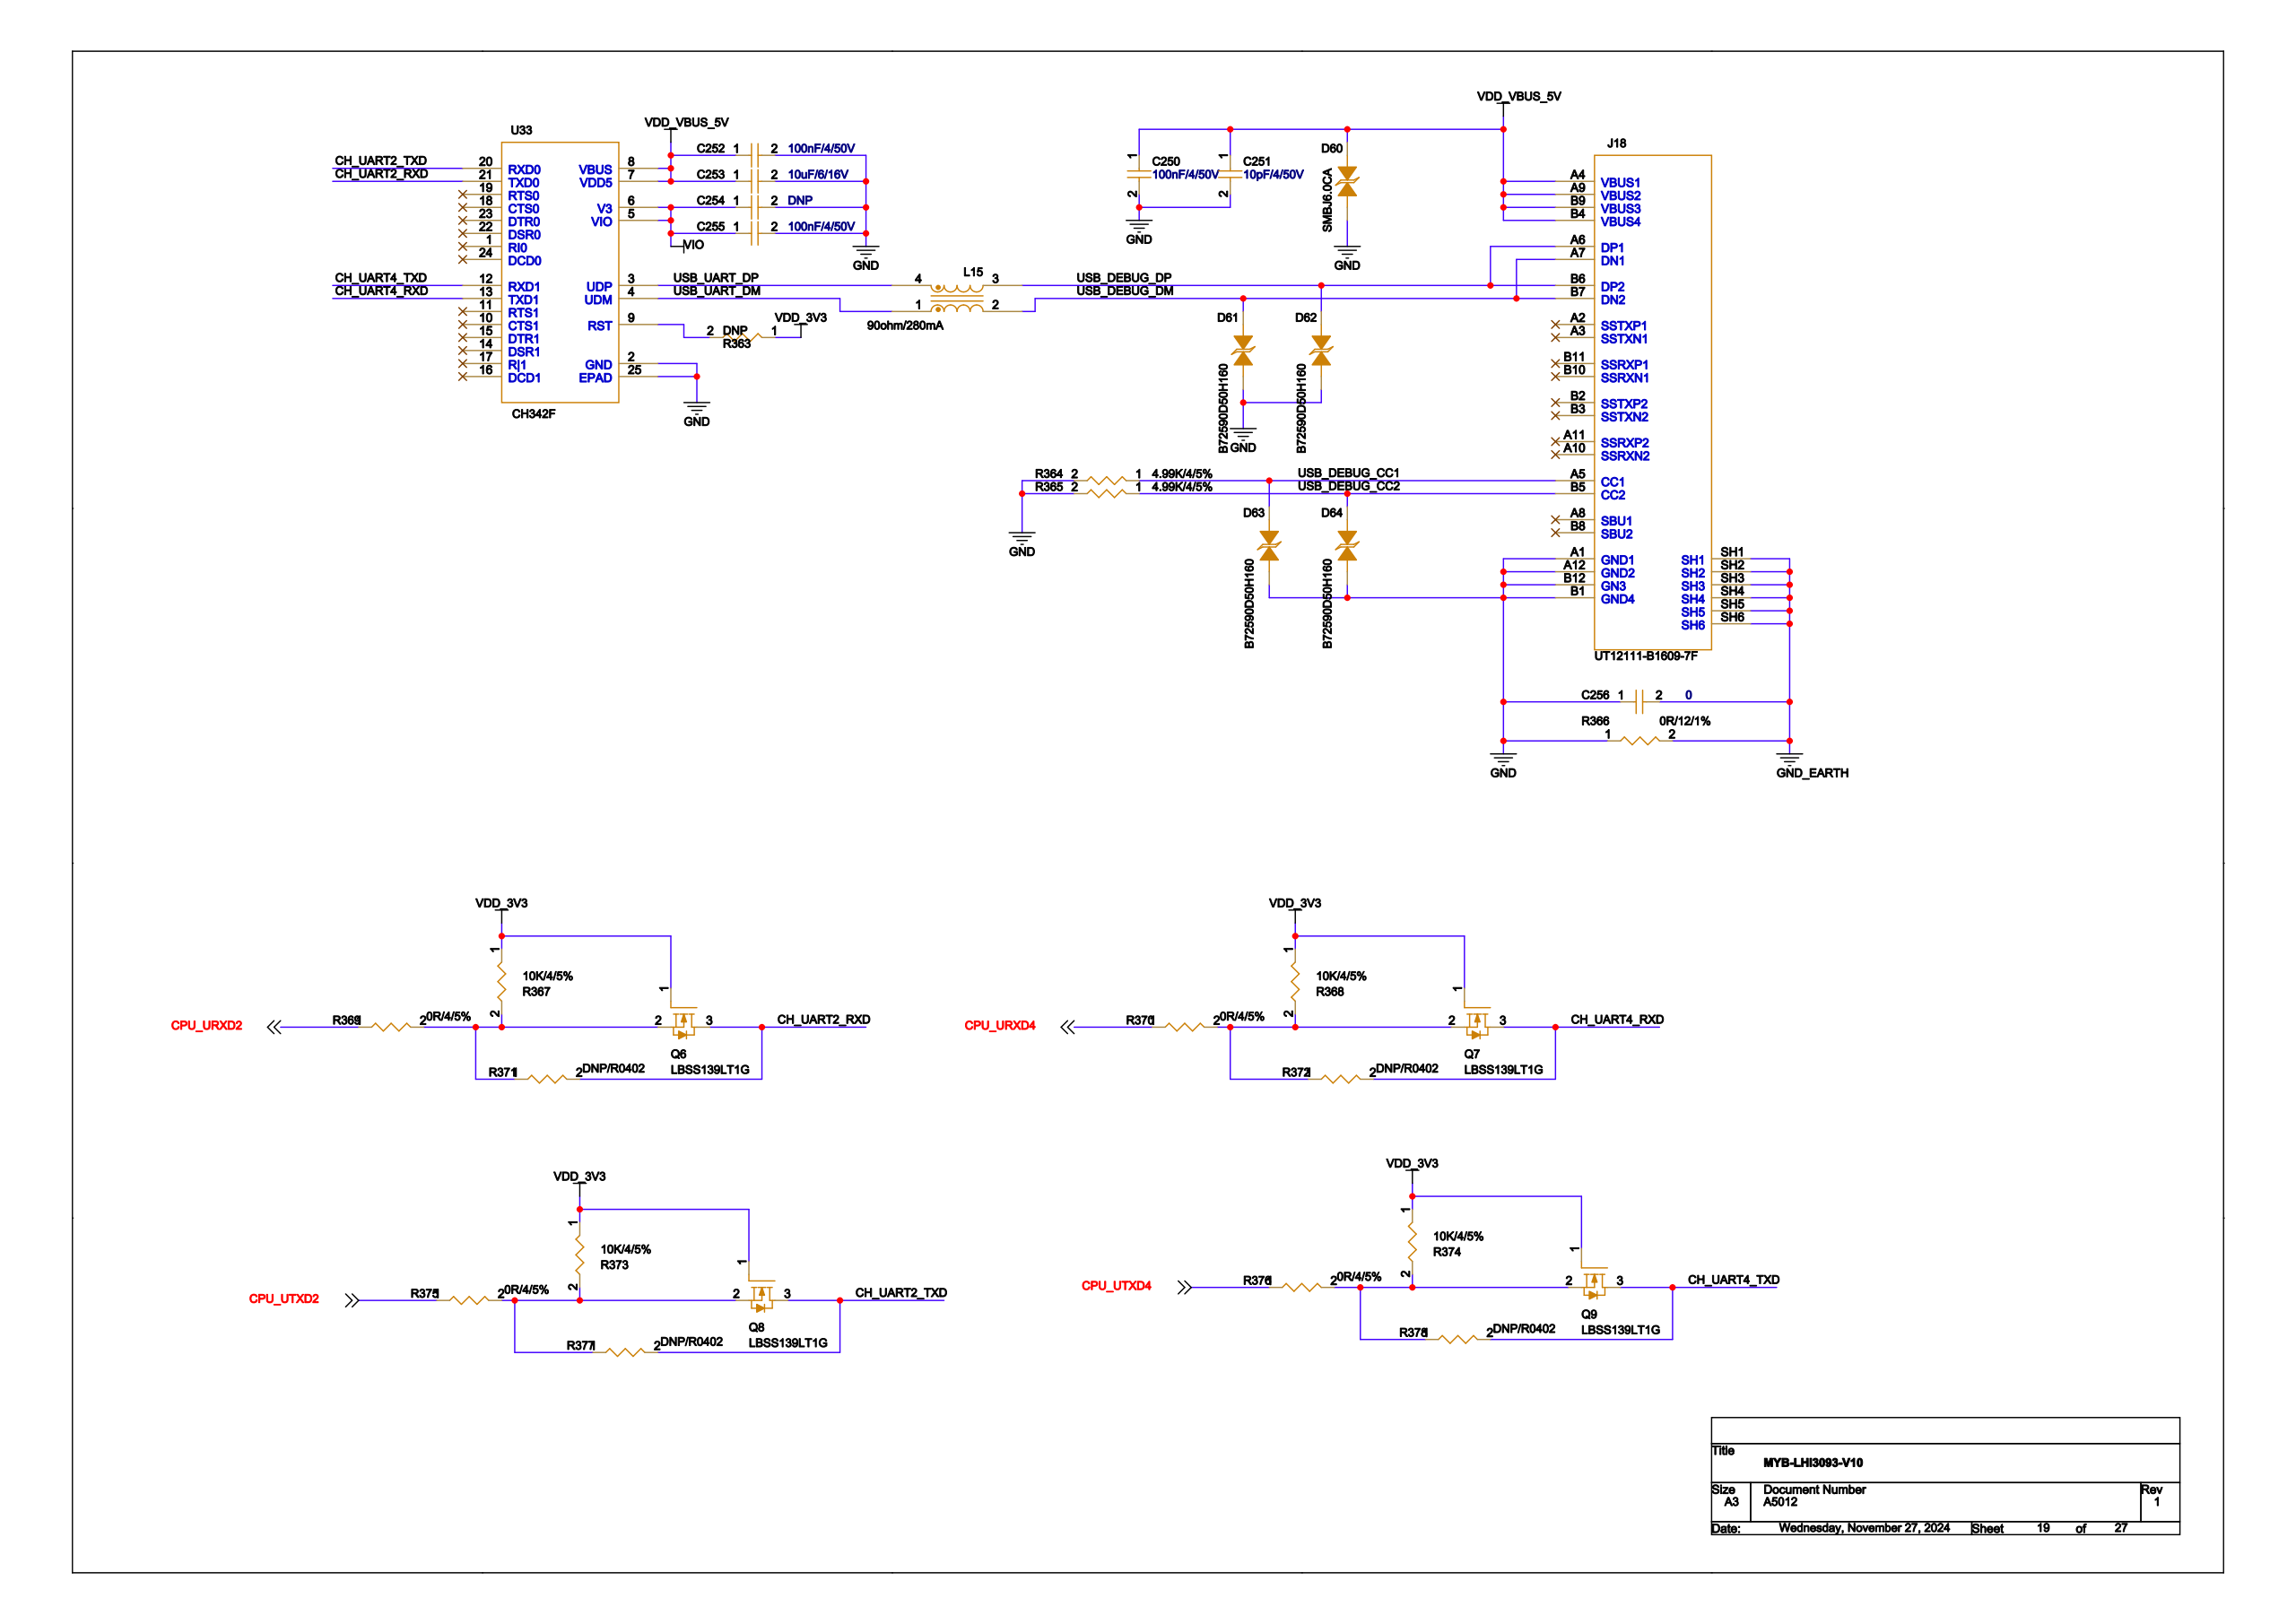Circuit board | Cadence Allegro | 1159 parts | 708 nets | one sheet of the schematic
Parts on this sheet (reference | value | footprint):
C250 | 100nF/4/50V | C0402
C251 | 10pF/4/50V | C0402
C252 | 100nF/4/50V | C0402
C253 | 10uF/6/16V | C0603
C254 | DNP | C0603
C255 | 100nF/4/50V | C0402
C256 | 0 | C1206
J18 | UT12111-B1609-7F | UT12111-B1609-7F
L15 | 90ohm/280mA | INDCM-SDCW2012
Q6 | LBSS139LT1G | SOT-23
Q7 | LBSS139LT1G | SOT-23
Q8 | LBSS139LT1G | SOT-23
Q9 | LBSS139LT1G | SOT-23
R363 | DNP | R0402
R364 | 4.99K/4/5% | R0402
R365 | 4.99K/4/5% | R0402
R366 | 0R/12/1% | R1206
R367 | 10K/4/5% | R0402
R368 | 10K/4/5% | R0402
R369 | 0R/4/5% | R0402
R370 | 0R/4/5% | R0402
R371 | DNP/R0402 | R0402
R372 | DNP/R0402 | R0402
R373 | 10K/4/5% | R0402
R374 | 10K/4/5% | R0402
R375 | 0R/4/5% | R0402
R376 | 0R/4/5% | R0402
R377 | DNP/R0402 | R0402
R378 | DNP/R0402 | R0402
U33 | CH342F | QFN24-0_5
Nets of these parts (net: part-pin ...):
GND: C250-2 C251-2 C252-2 C253-2 C254-2 C255-2 C256-1 J18-A1 J18-A12 J18-B1 J18-B12 R364-2 R365-2 R366-1 U33-2 U33-25
VDD_3V3: Q6-1 Q7-1 Q8-1 Q9-1 R363-1 R367-1 R368-1 R373-1 R374-1
VDD_VBUS_5V: C250-1 C251-1 C252-1 C253-1 J18-A4 J18-A9 J18-B4 J18-B9 U33-7 U33-8
VIO: C254-1 C255-1 U33-5 U33-6
GND_EARTH: C256-2 J18-SH1 J18-SH2 J18-SH3 J18-SH4 J18-SH5 J18-SH6 R366-2
USB_DEBUG_DM: J18-A7 J18-B7 L15-2
USB_DEBUG_DP: J18-A6 J18-B6 L15-3
USB_DEBUG_CC1: J18-A5 R364-1
USB_DEBUG_CC2: J18-B5 R365-1
USB_UART_DM: L15-1 U33-4
USB_UART_DP: L15-4 U33-3
CH_UART2_RXD: Q6-3 R371-2 U33-21
N15046704: Q6-2 R367-2 R369-2 R371-1
CH_UART4_RXD: Q7-3 R372-2 U33-13
N15047209: Q7-2 R368-2 R370-2 R372-1
CH_UART2_TXD: Q8-3 R377-2 U33-20
N15047550: Q8-2 R373-2 R375-2 R377-1
CH_UART4_TXD: Q9-3 R378-2 U33-12
N15047909: Q9-2 R374-2 R376-2 R378-1
CPU_URXD2: R369-1
CPU_URXD4: R370-1
CPU_UTXD2: R375-1
CPU_UTXD4: R376-1
N15043643: R363-2 U33-9